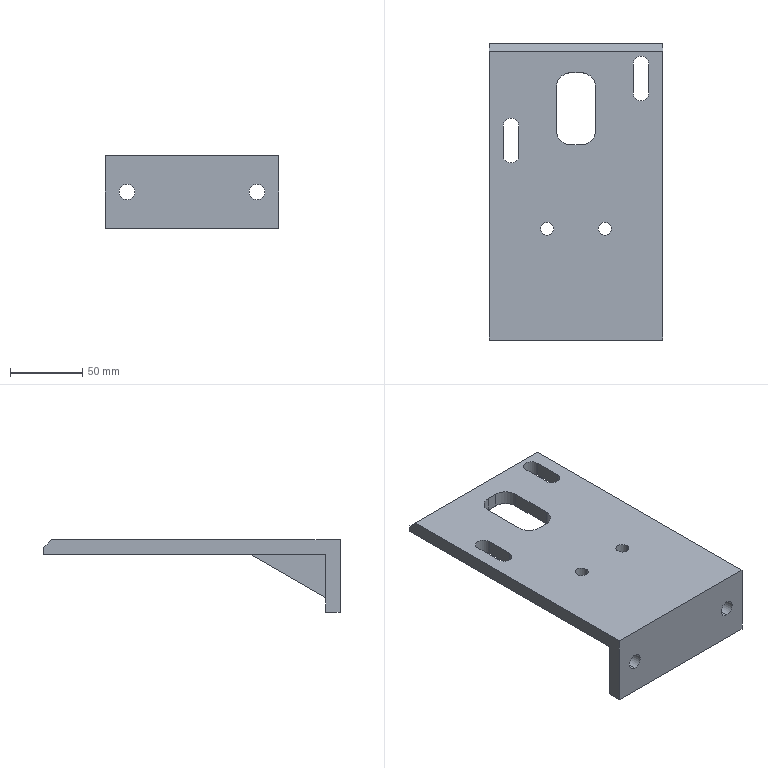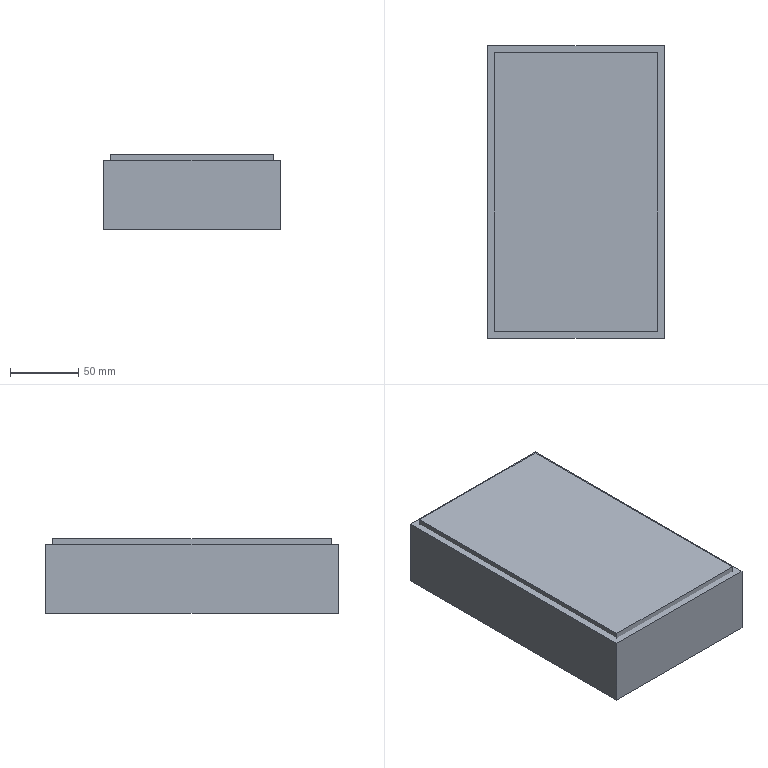CAM job | NX | 3+2 milling | part box 120 x 205 x 50 mm | stock box 130 x 215 x 55 mm
Tools:
number,name,description,diameter,corner_radius,flute_length,length,flutes
19,D80,Milling Tool-5 Parameters,80.0,0.0,50.0,75.0,2
15,D10,Milling Tool-5 Parameters,10.0,0.0,50.0,75.0,2
14,D10JING,Milling Tool-5 Parameters,10.0,0.0,50.0,75.0,2
12,D6,Milling Tool-5 Parameters,6.0,0.0,50.0,75.0,2
1,D6A45,Milling Tool-5 Parameters,6.0,0.0,50.0,75.0,2
17,D4R0.5,Milling Tool-5 Parameters,4.0,0.5,50.0,75.0,2
16,D8R0.5,Milling Tool-5 Parameters,8.0,0.5,50.0,75.0,2
Operations:
program,operation,operation_type,tool,method,geometry_group,spindle_rpm,surface_speed,feed_per_tooth,feed_cut,feed_plunge,cut_length_mm,path_length_mm,cut_time_min,machine_time_min
1,FLOOR_WALL,VolumeBased25DMillingOperation,D80,METHOD,A,6500.0,1633.0,0.1154,1500.0,100.0,994.997,1048.997,0.6633,0.6687
1,ZLEVEL_PROFILE,ZLevelMilling,D10,METHOD,A,9500.0,298.0,0.1316,2500.0,100.0,36205.981,36312.981,14.482,14.493
1,ZLEVEL_PROFILE_COPY,ZLevelMilling,D10,METHOD,A,9500.0,298.0,0.1316,2500.0,100.0,1012.043,1242.27,0.4048,0.4278
1,PLANAR_MILL,PlanarMilling,D10,METHOD,A,9500.0,298.0,0.1316,2500.0,1000.0,2180.648,2958.316,1.158,1.236
1,ZLEVEL_PROFILE_COPY_1_COPY_COPY_1,ZLevelMilling,D10JING,METHOD,A,9500.0,298.0,0.0632,1200.0,1000.0,2066.263,2446.982,1.724,1.762
1,ZLEVEL_PROFILE_COPY_1_COPY_COPY_1_COPY,ZLevelMilling,D6,METHOD,A,9500.0,298.0,0.0632,1200.0,1000.0,245.368,674.208,0.2058,0.2487
1,HOLE_MILLING,CylinderMilling,D6,METHOD,A,9500.0,179.0,0.0868,1650.0,100.0,396.437,575.437,0.2403,0.2582
1,ZLEVEL_PROFILE_1,ZLevelMilling,D4R0.5,METHOD,A,9500.0,119.0,0.1842,3500.0,1000.0,18891.164,19022.969,5.401,5.414
1,PLANAR_MILL_COPY_COPY_COPY_COPY_COPY_COPY_1,PlanarMilling,D6A45,METHOD,A,9500.0,179.0,0.0658,1250.0,100.0,1000.442,1592.685,0.8004,0.8596
1,刀补6,CylinderMilling,D6,METHOD,A,9500.0,179.0,0.0526,1000.0,100.0,125.337,304.337,0.1253,0.1432
2,FLOOR_WALL_COPY,VolumeBased25DMillingOperation,D80,METHOD,B,6500.0,1633.0,0.1154,1500.0,100.0,4794.985,6276.366,3.197,3.345
2,FLOOR_WALL_1,VolumeBased25DMillingOperation,D10,METHOD,B,9500.0,298.0,0.1842,3500.0,1000.0,193526.516,196238.725,55.566,55.837
2,FLOOR_WALL_1_COPY,VolumeBased25DMillingOperation,D10JING,METHOD,B,9500.0,298.0,0.0632,1200.0,1000.0,5321.632,5660.26,4.436,4.47
2,ZLEVEL_PROFILE_COPY_1_COPY_COPY_1_COPY_1,ZLevelMilling,D10JING,METHOD,B,9500.0,298.0,0.0632,1200.0,1000.0,137.645,215.445,0.1153,0.1231
2,ZLEVEL_PROFILE_COPY_1_COPY_COPY_1_COPY_1_COPY,ZLevelMilling,D10JING,METHOD,B,9500.0,298.0,0.0632,1200.0,1000.0,562.181,1601.796,0.4721,0.5761
2,ZLEVEL_PROFILE_1_COPY,ZLevelMilling,D8R0.5,METHOD,B,9500.0,119.0,0.1842,3500.0,1000.0,13235.576,13515.161,3.787,3.815
2,ZLEVEL_PROFILE_COPY_1,ZLevelMilling,D6,METHOD,B,5000.0,94.0,0.1,1000.0,100.0,2649.959,4081.686,2.65,2.793
2,PLANAR_MILL_COPY_COPY_COPY_COPY_COPY_COPY_1_COPY,PlanarMilling,D6A45,METHOD,B,9500.0,179.0,0.0658,1250.0,100.0,270.749,329.749,0.2166,0.2225
2,PLANAR_MILL_COPY_COPY_COPY_COPY_COPY_COPY_1_COPY_COPY,PlanarMilling,D6A45,METHOD,B,9500.0,179.0,0.0658,1250.0,100.0,863.146,2075.23,0.6905,0.8117
3,HOLE_MILLING_COPY_1,CylinderMilling,D6,METHOD,C,9500.0,179.0,0.0868,1650.0,100.0,678.932,907.932,0.4115,0.4344
3,PLANAR_MILL_COPY_COPY_COPY_COPY_COPY_COPY_1_COPY_1,PlanarMilling,D6A45,METHOD,C,9500.0,179.0,0.0658,1250.0,100.0,72.75,286.891,0.0582,0.0796
3,刀补,CylinderMilling,D6,METHOD,C,9500.0,179.0,0.0526,1000.0,100.0,209.26,438.26,0.2093,0.2322